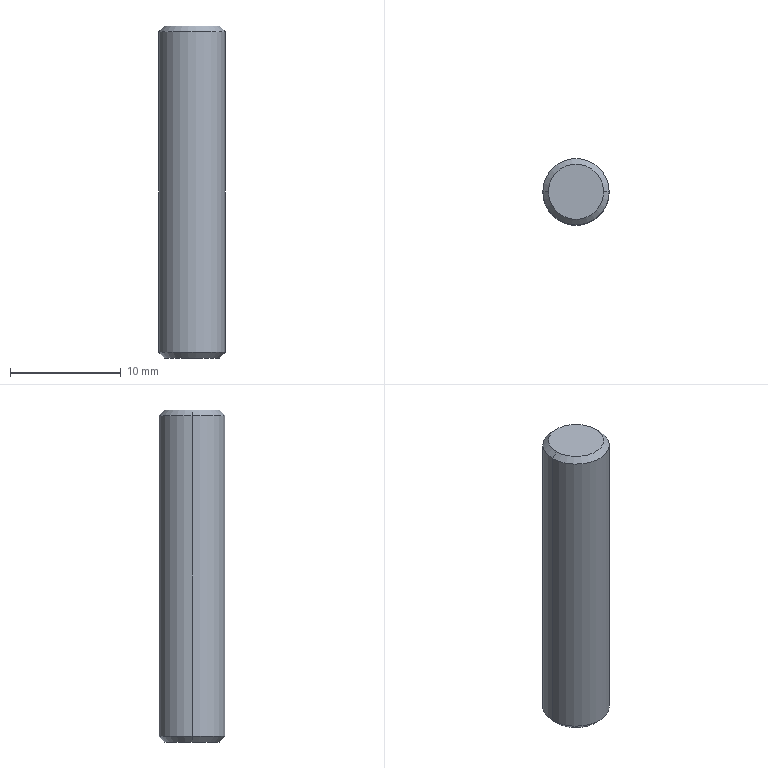Part | SolidWorks | features Chamfer 1, Extrusion 1 | 1 solid | 8 faces | box 6 x 6 x 30 mm | volume 843.779 mm3 | cone 4 | cylinder 2 | plane 2 | commonest cylinder face diameters 6 x2
STEP:
#1=CARTESIAN_POINT('',(2.5,0.,30.));
#2=VERTEX_POINT('',#1);
#3=CARTESIAN_POINT('',(-2.5,0.,30.));
#4=VERTEX_POINT('',#3);
#5=CARTESIAN_POINT('',(0.,0.,30.));
#6=DIRECTION('',(0.,0.,1.));
#7=DIRECTION('',(1.,0.,0.));
#8=AXIS2_PLACEMENT_3D('',#5,#6,#7);
#9=CIRCLE('',#8,2.5);
#10=EDGE_CURVE('',#2,#4,#9,.T.);
#11=ORIENTED_EDGE('',*,*,#10,.F.);
#12=CARTESIAN_POINT('',(3.,0.,29.5));
#13=VERTEX_POINT('',#12);
#14=CARTESIAN_POINT('',(2.5,0.,30.));
#15=DIRECTION('',(0.7071,0.,-0.7071));
#16=VECTOR('',#15,1000.);
#17=LINE('',#14,#16);
#18=EDGE_CURVE('',#2,#13,#17,.T.);
#19=ORIENTED_EDGE('',*,*,#18,.T.);
#20=CARTESIAN_POINT('',(-3.,0.,29.5));
#21=VERTEX_POINT('',#20);
#22=CARTESIAN_POINT('',(0.,0.,29.5));
#23=DIRECTION('',(0.,0.,-1.));
#24=DIRECTION('',(1.,0.,0.));
#25=AXIS2_PLACEMENT_3D('',#22,#23,#24);
#26=CIRCLE('',#25,3.);
#27=EDGE_CURVE('',#21,#13,#26,.T.);
#28=ORIENTED_EDGE('',*,*,#27,.F.);
#29=CARTESIAN_POINT('',(-2.5,0.,30.));
#30=DIRECTION('',(-0.7071,0.,-0.7071));
#31=VECTOR('',#30,1000.);
#32=LINE('',#29,#31);
#33=EDGE_CURVE('',#4,#21,#32,.T.);
#34=ORIENTED_EDGE('',*,*,#33,.F.);
#35=EDGE_LOOP('',(#11,#19,#28,#34));
#36=FACE_OUTER_BOUND('',#35,.T.);
#37=CARTESIAN_POINT('',(0.,0.,30.));
#38=DIRECTION('',(0.,0.,-1.));
#39=DIRECTION('',(-1.,0.,0.));
#40=AXIS2_PLACEMENT_3D('',#37,#38,#39);
#41=CONICAL_SURFACE('',#40,2.5,0.7854);
#42=ADVANCED_FACE('',(#36),#41,.T.);
#43=CARTESIAN_POINT('',(-2.5,0.,0.));
#44=VERTEX_POINT('',#43);
#45=CARTESIAN_POINT('',(2.5,0.,0.));
#46=VERTEX_POINT('',#45);
#47=CARTESIAN_POINT('',(0.,0.,0.));
#48=DIRECTION('',(0.,0.,-1.));
#49=DIRECTION('',(1.,0.,0.));
#50=AXIS2_PLACEMENT_3D('',#47,#48,#49);
#51=CIRCLE('',#50,2.5);
#52=EDGE_CURVE('',#44,#46,#51,.T.);
#53=ORIENTED_EDGE('',*,*,#52,.F.);
#54=CARTESIAN_POINT('',(-3.,0.,0.5));
#55=VERTEX_POINT('',#54);
#56=CARTESIAN_POINT('',(-3.,0.,0.5));
#57=DIRECTION('',(-0.7071,0.,0.7071));
#58=VECTOR('',#57,1000.);
#59=LINE('',#56,#58);
#60=EDGE_CURVE('',#44,#55,#59,.T.);
#61=ORIENTED_EDGE('',*,*,#60,.T.);
#62=CARTESIAN_POINT('',(3.,0.,0.5));
#63=VERTEX_POINT('',#62);
#64=CARTESIAN_POINT('',(0.,0.,0.5));
#65=DIRECTION('',(0.,0.,1.));
#66=DIRECTION('',(1.,0.,0.));
#67=AXIS2_PLACEMENT_3D('',#64,#65,#66);
#68=CIRCLE('',#67,3.);
#69=EDGE_CURVE('',#63,#55,#68,.T.);
#70=ORIENTED_EDGE('',*,*,#69,.F.);
#71=CARTESIAN_POINT('',(3.,0.,0.5));
#72=DIRECTION('',(0.7071,0.,0.7071));
#73=VECTOR('',#72,1000.);
#74=LINE('',#71,#73);
#75=EDGE_CURVE('',#46,#63,#74,.T.);
#76=ORIENTED_EDGE('',*,*,#75,.F.);
#77=EDGE_LOOP('',(#53,#61,#70,#76));
#78=FACE_OUTER_BOUND('',#77,.T.);
#79=CARTESIAN_POINT('',(0.,0.,0.5));
#80=DIRECTION('',(0.,0.,1.));
#81=DIRECTION('',(1.,0.,0.));
#82=AXIS2_PLACEMENT_3D('',#79,#80,#81);
#83=CONICAL_SURFACE('',#82,3.,0.7854);
#84=ADVANCED_FACE('',(#78),#83,.T.);
#85=ORIENTED_EDGE('',*,*,#27,.T.);
#86=CARTESIAN_POINT('',(3.,0.,30.));
#87=DIRECTION('',(0.,0.,-1.));
#88=VECTOR('',#87,1000.);
#89=LINE('',#86,#88);
#90=EDGE_CURVE('',#13,#63,#89,.T.);
#91=ORIENTED_EDGE('',*,*,#90,.T.);
#92=ORIENTED_EDGE('',*,*,#69,.T.);
#93=CARTESIAN_POINT('',(-3.,0.,30.));
#94=DIRECTION('',(0.,0.,-1.));
#95=VECTOR('',#94,1000.);
#96=LINE('',#93,#95);
#97=EDGE_CURVE('',#21,#55,#96,.T.);
#98=ORIENTED_EDGE('',*,*,#97,.F.);
#99=EDGE_LOOP('',(#85,#91,#92,#98));
#100=FACE_OUTER_BOUND('',#99,.T.);
#101=CARTESIAN_POINT('',(0.,0.,30.));
#102=DIRECTION('',(0.,0.,-1.));
#103=DIRECTION('',(-1.,0.,0.));
#104=AXIS2_PLACEMENT_3D('',#101,#102,#103);
#105=CYLINDRICAL_SURFACE('',#104,3.);
#106=ADVANCED_FACE('',(#100),#105,.T.);
#107=ORIENTED_EDGE('',*,*,#90,.F.);
#108=CARTESIAN_POINT('',(0.,0.,29.5));
#109=DIRECTION('',(0.,0.,-1.));
#110=DIRECTION('',(1.,0.,0.));
#111=AXIS2_PLACEMENT_3D('',#108,#109,#110);
#112=CIRCLE('',#111,3.);
#113=EDGE_CURVE('',#13,#21,#112,.T.);
#114=ORIENTED_EDGE('',*,*,#113,.T.);
#115=ORIENTED_EDGE('',*,*,#97,.T.);
#116=CARTESIAN_POINT('',(0.,0.,0.5));
#117=DIRECTION('',(0.,0.,1.));
#118=DIRECTION('',(1.,0.,0.));
#119=AXIS2_PLACEMENT_3D('',#116,#117,#118);
#120=CIRCLE('',#119,3.);
#121=EDGE_CURVE('',#55,#63,#120,.T.);
#122=ORIENTED_EDGE('',*,*,#121,.T.);
#123=EDGE_LOOP('',(#107,#114,#115,#122));
#124=FACE_OUTER_BOUND('',#123,.T.);
#125=CARTESIAN_POINT('',(0.,0.,30.));
#126=DIRECTION('',(0.,0.,-1.));
#127=DIRECTION('',(-1.,0.,0.));
#128=AXIS2_PLACEMENT_3D('',#125,#126,#127);
#129=CYLINDRICAL_SURFACE('',#128,3.);
#130=ADVANCED_FACE('',(#124),#129,.T.);
#131=CARTESIAN_POINT('',(0.,0.,30.));
#132=DIRECTION('',(0.,0.,1.));
#133=DIRECTION('',(1.,0.,0.));
#134=AXIS2_PLACEMENT_3D('',#131,#132,#133);
#135=CIRCLE('',#134,2.5);
#136=EDGE_CURVE('',#4,#2,#135,.T.);
#137=ORIENTED_EDGE('',*,*,#136,.T.);
#138=ORIENTED_EDGE('',*,*,#10,.T.);
#139=EDGE_LOOP('',(#137,#138));
#140=FACE_OUTER_BOUND('',#139,.T.);
#141=CARTESIAN_POINT('',(0.,0.,30.));
#142=DIRECTION('',(0.,0.,1.));
#143=DIRECTION('',(1.,0.,0.));
#144=AXIS2_PLACEMENT_3D('',#141,#142,#143);
#145=PLANE('',#144);
#146=ADVANCED_FACE('',(#140),#145,.T.);
#147=CARTESIAN_POINT('',(0.,0.,0.));
#148=DIRECTION('',(0.,0.,-1.));
#149=DIRECTION('',(1.,0.,0.));
#150=AXIS2_PLACEMENT_3D('',#147,#148,#149);
#151=CIRCLE('',#150,2.5);
#152=EDGE_CURVE('',#46,#44,#151,.T.);
#153=ORIENTED_EDGE('',*,*,#152,.T.);
#154=ORIENTED_EDGE('',*,*,#52,.T.);
#155=EDGE_LOOP('',(#153,#154));
#156=FACE_OUTER_BOUND('',#155,.T.);
#157=CARTESIAN_POINT('',(0.,0.,0.));
#158=DIRECTION('',(0.,0.,1.));
#159=DIRECTION('',(1.,0.,0.));
#160=AXIS2_PLACEMENT_3D('',#157,#158,#159);
#161=PLANE('',#160);
#162=ADVANCED_FACE('',(#156),#161,.F.);
#163=ORIENTED_EDGE('',*,*,#60,.F.);
#164=ORIENTED_EDGE('',*,*,#152,.F.);
#165=ORIENTED_EDGE('',*,*,#75,.T.);
#166=ORIENTED_EDGE('',*,*,#121,.F.);
#167=EDGE_LOOP('',(#163,#164,#165,#166));
#168=FACE_OUTER_BOUND('',#167,.T.);
#169=CARTESIAN_POINT('',(0.,0.,0.5));
#170=DIRECTION('',(0.,0.,1.));
#171=DIRECTION('',(1.,0.,0.));
#172=AXIS2_PLACEMENT_3D('',#169,#170,#171);
#173=CONICAL_SURFACE('',#172,3.,0.7854);
#174=ADVANCED_FACE('',(#168),#173,.T.);
#175=ORIENTED_EDGE('',*,*,#18,.F.);
#176=ORIENTED_EDGE('',*,*,#136,.F.);
#177=ORIENTED_EDGE('',*,*,#33,.T.);
#178=ORIENTED_EDGE('',*,*,#113,.F.);
#179=EDGE_LOOP('',(#175,#176,#177,#178));
#180=FACE_OUTER_BOUND('',#179,.T.);
#181=CARTESIAN_POINT('',(0.,0.,30.));
#182=DIRECTION('',(0.,0.,-1.));
#183=DIRECTION('',(-1.,0.,0.));
#184=AXIS2_PLACEMENT_3D('',#181,#182,#183);
#185=CONICAL_SURFACE('',#184,2.5,0.7854);
#186=ADVANCED_FACE('',(#180),#185,.T.);
#187=CLOSED_SHELL('',(#42,#84,#106,#130,#146,#162,#174,#186));
#188=MANIFOLD_SOLID_BREP('',#187);
#189=CARTESIAN_POINT('',(0.,0.,0.));
#190=DIRECTION('',(0.,0.,1.));
#191=DIRECTION('',(1.,0.,0.));
#192=AXIS2_PLACEMENT_3D('',#189,#190,#191);
#193=(LENGTH_UNIT()NAMED_UNIT(*)SI_UNIT(.MILLI.,.METRE.));
#194=UNCERTAINTY_MEASURE_WITH_UNIT(LENGTH_MEASURE(0.00001),#193,'','');
#195=(NAMED_UNIT(*)PLANE_ANGLE_UNIT()SI_UNIT($,.RADIAN.));
#196=(NAMED_UNIT(*)SI_UNIT($,.STERADIAN.)SOLID_ANGLE_UNIT());
#197=(GEOMETRIC_REPRESENTATION_CONTEXT(3)GLOBAL_UNCERTAINTY_ASSIGNED_CONTEXT((#194))GLOBAL_UNIT_ASSIGNED_CONTEXT((#193,#195,#196))REPRESENTATION_CONTEXT('',''));
#198=ADVANCED_BREP_SHAPE_REPRESENTATION('',(#188,#192),#197);